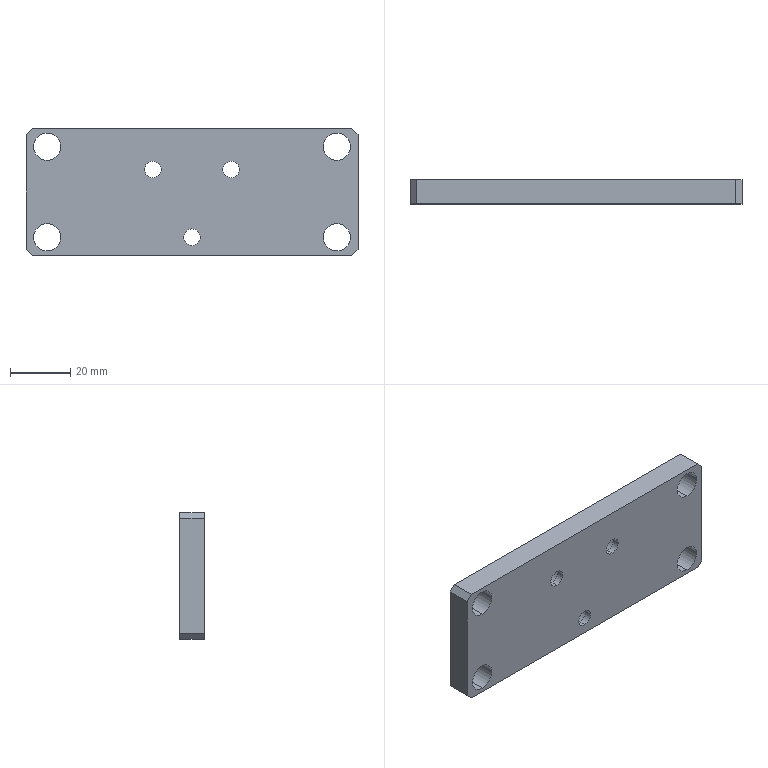Part | SolidWorks | features HoleWzd 2, MirrorPattern 2, Chamfer 1, Extrusion 1 | 1 solid | 33 faces | box 110 x 8 x 42 mm | volume 33353 mm3 | cylinder 20 | plane 13 | commonest cylinder face diameters 9 x8 5.5 x6 10 x6
STEP:
#1=CARTESIAN_POINT('',(-48.,4.,-10.5));
#2=VERTEX_POINT('',#1);
#3=CARTESIAN_POINT('',(-48.,4.,-19.5));
#4=VERTEX_POINT('',#3);
#5=CARTESIAN_POINT('',(-48.,4.,-15.));
#6=DIRECTION('',(0.,-1.,0.));
#7=DIRECTION('',(0.,0.,-1.));
#8=AXIS2_PLACEMENT_3D('',#5,#6,#7);
#9=CIRCLE('',#8,4.5);
#10=EDGE_CURVE('',#2,#4,#9,.T.);
#11=ORIENTED_EDGE('',*,*,#10,.F.);
#12=CARTESIAN_POINT('',(-48.,-4.,-10.5));
#13=VERTEX_POINT('',#12);
#14=CARTESIAN_POINT('',(-48.,-4.,-10.5));
#15=DIRECTION('',(0.,-1.,0.));
#16=VECTOR('',#15,1000.);
#17=LINE('',#14,#16);
#18=EDGE_CURVE('',#2,#13,#17,.T.);
#19=ORIENTED_EDGE('',*,*,#18,.T.);
#20=CARTESIAN_POINT('',(-48.,-4.,-19.5));
#21=VERTEX_POINT('',#20);
#22=CARTESIAN_POINT('',(-48.,-4.,-15.));
#23=DIRECTION('',(0.,-1.,0.));
#24=DIRECTION('',(0.,0.,-1.));
#25=AXIS2_PLACEMENT_3D('',#22,#23,#24);
#26=CIRCLE('',#25,4.5);
#27=EDGE_CURVE('',#13,#21,#26,.T.);
#28=ORIENTED_EDGE('',*,*,#27,.T.);
#29=CARTESIAN_POINT('',(-48.,-4.,-19.5));
#30=DIRECTION('',(0.,-1.,0.));
#31=VECTOR('',#30,1000.);
#32=LINE('',#29,#31);
#33=EDGE_CURVE('',#4,#21,#32,.T.);
#34=ORIENTED_EDGE('',*,*,#33,.F.);
#35=EDGE_LOOP('',(#11,#19,#28,#34));
#36=FACE_OUTER_BOUND('',#35,.T.);
#37=CARTESIAN_POINT('',(-48.,-4.,-15.));
#38=DIRECTION('',(0.,-1.,0.));
#39=DIRECTION('',(0.,0.,-1.));
#40=AXIS2_PLACEMENT_3D('',#37,#38,#39);
#41=CYLINDRICAL_SURFACE('',#40,4.5);
#42=ADVANCED_FACE('',(#36),#41,.F.);
#43=CARTESIAN_POINT('',(-48.,4.,19.5));
#44=VERTEX_POINT('',#43);
#45=CARTESIAN_POINT('',(-48.,4.,10.5));
#46=VERTEX_POINT('',#45);
#47=CARTESIAN_POINT('',(-48.,4.,15.));
#48=DIRECTION('',(0.,-1.,0.));
#49=DIRECTION('',(0.,0.,-1.));
#50=AXIS2_PLACEMENT_3D('',#47,#48,#49);
#51=CIRCLE('',#50,4.5);
#52=EDGE_CURVE('',#44,#46,#51,.T.);
#53=ORIENTED_EDGE('',*,*,#52,.F.);
#54=CARTESIAN_POINT('',(-48.,-4.,19.5));
#55=VERTEX_POINT('',#54);
#56=CARTESIAN_POINT('',(-48.,-4.,19.5));
#57=DIRECTION('',(0.,-1.,0.));
#58=VECTOR('',#57,1000.);
#59=LINE('',#56,#58);
#60=EDGE_CURVE('',#44,#55,#59,.T.);
#61=ORIENTED_EDGE('',*,*,#60,.T.);
#62=CARTESIAN_POINT('',(-48.,-4.,10.5));
#63=VERTEX_POINT('',#62);
#64=CARTESIAN_POINT('',(-48.,-4.,15.));
#65=DIRECTION('',(0.,-1.,0.));
#66=DIRECTION('',(0.,0.,-1.));
#67=AXIS2_PLACEMENT_3D('',#64,#65,#66);
#68=CIRCLE('',#67,4.5);
#69=EDGE_CURVE('',#55,#63,#68,.T.);
#70=ORIENTED_EDGE('',*,*,#69,.T.);
#71=CARTESIAN_POINT('',(-48.,-4.,10.5));
#72=DIRECTION('',(0.,-1.,0.));
#73=VECTOR('',#72,1000.);
#74=LINE('',#71,#73);
#75=EDGE_CURVE('',#46,#63,#74,.T.);
#76=ORIENTED_EDGE('',*,*,#75,.F.);
#77=EDGE_LOOP('',(#53,#61,#70,#76));
#78=FACE_OUTER_BOUND('',#77,.T.);
#79=CARTESIAN_POINT('',(-48.,-4.,15.));
#80=DIRECTION('',(0.,-1.,0.));
#81=DIRECTION('',(0.,0.,-1.));
#82=AXIS2_PLACEMENT_3D('',#79,#80,#81);
#83=CYLINDRICAL_SURFACE('',#82,4.5);
#84=ADVANCED_FACE('',(#78),#83,.F.);
#85=CARTESIAN_POINT('',(48.,4.,-10.5));
#86=VERTEX_POINT('',#85);
#87=CARTESIAN_POINT('',(48.,4.,-19.5));
#88=VERTEX_POINT('',#87);
#89=CARTESIAN_POINT('',(48.,4.,-15.));
#90=DIRECTION('',(0.,-1.,0.));
#91=DIRECTION('',(0.,0.,-1.));
#92=AXIS2_PLACEMENT_3D('',#89,#90,#91);
#93=CIRCLE('',#92,4.5);
#94=EDGE_CURVE('',#86,#88,#93,.T.);
#95=ORIENTED_EDGE('',*,*,#94,.F.);
#96=CARTESIAN_POINT('',(48.,-4.,-10.5));
#97=VERTEX_POINT('',#96);
#98=CARTESIAN_POINT('',(48.,-4.,-10.5));
#99=DIRECTION('',(0.,-1.,0.));
#100=VECTOR('',#99,1000.);
#101=LINE('',#98,#100);
#102=EDGE_CURVE('',#86,#97,#101,.T.);
#103=ORIENTED_EDGE('',*,*,#102,.T.);
#104=CARTESIAN_POINT('',(48.,-4.,-19.5));
#105=VERTEX_POINT('',#104);
#106=CARTESIAN_POINT('',(48.,-4.,-15.));
#107=DIRECTION('',(0.,-1.,0.));
#108=DIRECTION('',(0.,0.,-1.));
#109=AXIS2_PLACEMENT_3D('',#106,#107,#108);
#110=CIRCLE('',#109,4.5);
#111=EDGE_CURVE('',#97,#105,#110,.T.);
#112=ORIENTED_EDGE('',*,*,#111,.T.);
#113=CARTESIAN_POINT('',(48.,-4.,-19.5));
#114=DIRECTION('',(0.,-1.,0.));
#115=VECTOR('',#114,1000.);
#116=LINE('',#113,#115);
#117=EDGE_CURVE('',#88,#105,#116,.T.);
#118=ORIENTED_EDGE('',*,*,#117,.F.);
#119=EDGE_LOOP('',(#95,#103,#112,#118));
#120=FACE_OUTER_BOUND('',#119,.T.);
#121=CARTESIAN_POINT('',(48.,-4.,-15.));
#122=DIRECTION('',(0.,-1.,0.));
#123=DIRECTION('',(0.,0.,-1.));
#124=AXIS2_PLACEMENT_3D('',#121,#122,#123);
#125=CYLINDRICAL_SURFACE('',#124,4.5);
#126=ADVANCED_FACE('',(#120),#125,.F.);
#127=CARTESIAN_POINT('',(48.,4.,19.5));
#128=VERTEX_POINT('',#127);
#129=CARTESIAN_POINT('',(48.,4.,10.5));
#130=VERTEX_POINT('',#129);
#131=CARTESIAN_POINT('',(48.,4.,15.));
#132=DIRECTION('',(0.,-1.,0.));
#133=DIRECTION('',(0.,0.,-1.));
#134=AXIS2_PLACEMENT_3D('',#131,#132,#133);
#135=CIRCLE('',#134,4.5);
#136=EDGE_CURVE('',#128,#130,#135,.T.);
#137=ORIENTED_EDGE('',*,*,#136,.F.);
#138=CARTESIAN_POINT('',(48.,-4.,19.5));
#139=VERTEX_POINT('',#138);
#140=CARTESIAN_POINT('',(48.,-4.,19.5));
#141=DIRECTION('',(0.,-1.,0.));
#142=VECTOR('',#141,1000.);
#143=LINE('',#140,#142);
#144=EDGE_CURVE('',#128,#139,#143,.T.);
#145=ORIENTED_EDGE('',*,*,#144,.T.);
#146=CARTESIAN_POINT('',(48.,-4.,10.5));
#147=VERTEX_POINT('',#146);
#148=CARTESIAN_POINT('',(48.,-4.,15.));
#149=DIRECTION('',(0.,-1.,0.));
#150=DIRECTION('',(0.,0.,-1.));
#151=AXIS2_PLACEMENT_3D('',#148,#149,#150);
#152=CIRCLE('',#151,4.5);
#153=EDGE_CURVE('',#139,#147,#152,.T.);
#154=ORIENTED_EDGE('',*,*,#153,.T.);
#155=CARTESIAN_POINT('',(48.,-4.,10.5));
#156=DIRECTION('',(0.,-1.,0.));
#157=VECTOR('',#156,1000.);
#158=LINE('',#155,#157);
#159=EDGE_CURVE('',#130,#147,#158,.T.);
#160=ORIENTED_EDGE('',*,*,#159,.F.);
#161=EDGE_LOOP('',(#137,#145,#154,#160));
#162=FACE_OUTER_BOUND('',#161,.T.);
#163=CARTESIAN_POINT('',(48.,-4.,15.));
#164=DIRECTION('',(0.,-1.,0.));
#165=DIRECTION('',(0.,0.,-1.));
#166=AXIS2_PLACEMENT_3D('',#163,#164,#165);
#167=CYLINDRICAL_SURFACE('',#166,4.5);
#168=ADVANCED_FACE('',(#162),#167,.F.);
#169=CARTESIAN_POINT('',(0.,-1.7,-20.));
#170=VERTEX_POINT('',#169);
#171=CARTESIAN_POINT('',(0.,-1.7,-10.));
#172=VERTEX_POINT('',#171);
#173=CARTESIAN_POINT('',(0.,-1.7,-15.));
#174=DIRECTION('',(0.,1.,0.));
#175=DIRECTION('',(0.,0.,1.));
#176=AXIS2_PLACEMENT_3D('',#173,#174,#175);
#177=CIRCLE('',#176,5.);
#178=EDGE_CURVE('',#170,#172,#177,.T.);
#179=ORIENTED_EDGE('',*,*,#178,.F.);
#180=CARTESIAN_POINT('',(0.,4.,-20.));
#181=VERTEX_POINT('',#180);
#182=CARTESIAN_POINT('',(0.,4.,-20.));
#183=DIRECTION('',(0.,1.,0.));
#184=VECTOR('',#183,1000.);
#185=LINE('',#182,#184);
#186=EDGE_CURVE('',#170,#181,#185,.T.);
#187=ORIENTED_EDGE('',*,*,#186,.T.);
#188=CARTESIAN_POINT('',(0.,4.,-10.));
#189=VERTEX_POINT('',#188);
#190=CARTESIAN_POINT('',(0.,4.,-15.));
#191=DIRECTION('',(0.,1.,0.));
#192=DIRECTION('',(0.,0.,1.));
#193=AXIS2_PLACEMENT_3D('',#190,#191,#192);
#194=CIRCLE('',#193,5.);
#195=EDGE_CURVE('',#181,#189,#194,.T.);
#196=ORIENTED_EDGE('',*,*,#195,.T.);
#197=CARTESIAN_POINT('',(0.,4.,-10.));
#198=DIRECTION('',(0.,1.,0.));
#199=VECTOR('',#198,1000.);
#200=LINE('',#197,#199);
#201=EDGE_CURVE('',#172,#189,#200,.T.);
#202=ORIENTED_EDGE('',*,*,#201,.F.);
#203=EDGE_LOOP('',(#179,#187,#196,#202));
#204=FACE_OUTER_BOUND('',#203,.T.);
#205=CARTESIAN_POINT('',(0.,4.,-15.));
#206=DIRECTION('',(0.,1.,0.));
#207=DIRECTION('',(0.,0.,1.));
#208=AXIS2_PLACEMENT_3D('',#205,#206,#207);
#209=CYLINDRICAL_SURFACE('',#208,5.);
#210=ADVANCED_FACE('',(#204),#209,.F.);
#211=CARTESIAN_POINT('',(0.,-4.,-17.75));
#212=VERTEX_POINT('',#211);
#213=CARTESIAN_POINT('',(0.,-4.,-12.25));
#214=VERTEX_POINT('',#213);
#215=CARTESIAN_POINT('',(0.,-4.,-15.));
#216=DIRECTION('',(0.,1.,0.));
#217=DIRECTION('',(0.,0.,1.));
#218=AXIS2_PLACEMENT_3D('',#215,#216,#217);
#219=CIRCLE('',#218,2.75);
#220=EDGE_CURVE('',#212,#214,#219,.T.);
#221=ORIENTED_EDGE('',*,*,#220,.F.);
#222=CARTESIAN_POINT('',(0.,-1.7,-17.75));
#223=VERTEX_POINT('',#222);
#224=CARTESIAN_POINT('',(0.,4.,-17.75));
#225=DIRECTION('',(0.,1.,0.));
#226=VECTOR('',#225,1000.);
#227=LINE('',#224,#226);
#228=EDGE_CURVE('',#212,#223,#227,.T.);
#229=ORIENTED_EDGE('',*,*,#228,.T.);
#230=CARTESIAN_POINT('',(0.,-1.7,-12.25));
#231=VERTEX_POINT('',#230);
#232=CARTESIAN_POINT('',(0.,-1.7,-15.));
#233=DIRECTION('',(0.,1.,0.));
#234=DIRECTION('',(0.,0.,1.));
#235=AXIS2_PLACEMENT_3D('',#232,#233,#234);
#236=CIRCLE('',#235,2.75);
#237=EDGE_CURVE('',#223,#231,#236,.T.);
#238=ORIENTED_EDGE('',*,*,#237,.T.);
#239=CARTESIAN_POINT('',(0.,4.,-12.25));
#240=DIRECTION('',(0.,1.,0.));
#241=VECTOR('',#240,1000.);
#242=LINE('',#239,#241);
#243=EDGE_CURVE('',#214,#231,#242,.T.);
#244=ORIENTED_EDGE('',*,*,#243,.F.);
#245=EDGE_LOOP('',(#221,#229,#238,#244));
#246=FACE_OUTER_BOUND('',#245,.T.);
#247=CARTESIAN_POINT('',(0.,4.,-15.));
#248=DIRECTION('',(0.,1.,0.));
#249=DIRECTION('',(0.,0.,1.));
#250=AXIS2_PLACEMENT_3D('',#247,#248,#249);
#251=CYLINDRICAL_SURFACE('',#250,2.75);
#252=ADVANCED_FACE('',(#246),#251,.F.);
#253=CARTESIAN_POINT('',(-12.99,-1.7,2.5));
#254=VERTEX_POINT('',#253);
#255=CARTESIAN_POINT('',(-12.99,-1.7,12.5));
#256=VERTEX_POINT('',#255);
#257=CARTESIAN_POINT('',(-12.99,-1.7,7.5));
#258=DIRECTION('',(0.,1.,0.));
#259=DIRECTION('',(0.,0.,1.));
#260=AXIS2_PLACEMENT_3D('',#257,#258,#259);
#261=CIRCLE('',#260,5.);
#262=EDGE_CURVE('',#254,#256,#261,.T.);
#263=ORIENTED_EDGE('',*,*,#262,.F.);
#264=CARTESIAN_POINT('',(-12.99,4.,2.5));
#265=VERTEX_POINT('',#264);
#266=CARTESIAN_POINT('',(-12.99,4.,2.5));
#267=DIRECTION('',(0.,1.,0.));
#268=VECTOR('',#267,1000.);
#269=LINE('',#266,#268);
#270=EDGE_CURVE('',#254,#265,#269,.T.);
#271=ORIENTED_EDGE('',*,*,#270,.T.);
#272=CARTESIAN_POINT('',(-12.99,4.,12.5));
#273=VERTEX_POINT('',#272);
#274=CARTESIAN_POINT('',(-12.99,4.,7.5));
#275=DIRECTION('',(0.,1.,0.));
#276=DIRECTION('',(0.,0.,1.));
#277=AXIS2_PLACEMENT_3D('',#274,#275,#276);
#278=CIRCLE('',#277,5.);
#279=EDGE_CURVE('',#265,#273,#278,.T.);
#280=ORIENTED_EDGE('',*,*,#279,.T.);
#281=CARTESIAN_POINT('',(-12.99,4.,12.5));
#282=DIRECTION('',(0.,1.,0.));
#283=VECTOR('',#282,1000.);
#284=LINE('',#281,#283);
#285=EDGE_CURVE('',#256,#273,#284,.T.);
#286=ORIENTED_EDGE('',*,*,#285,.F.);
#287=EDGE_LOOP('',(#263,#271,#280,#286));
#288=FACE_OUTER_BOUND('',#287,.T.);
#289=CARTESIAN_POINT('',(-12.99,4.,7.5));
#290=DIRECTION('',(0.,1.,0.));
#291=DIRECTION('',(0.,0.,1.));
#292=AXIS2_PLACEMENT_3D('',#289,#290,#291);
#293=CYLINDRICAL_SURFACE('',#292,5.);
#294=ADVANCED_FACE('',(#288),#293,.F.);
#295=CARTESIAN_POINT('',(-12.99,-4.,4.75));
#296=VERTEX_POINT('',#295);
#297=CARTESIAN_POINT('',(-12.99,-4.,10.25));
#298=VERTEX_POINT('',#297);
#299=CARTESIAN_POINT('',(-12.99,-4.,7.5));
#300=DIRECTION('',(0.,1.,0.));
#301=DIRECTION('',(0.,0.,1.));
#302=AXIS2_PLACEMENT_3D('',#299,#300,#301);
#303=CIRCLE('',#302,2.75);
#304=EDGE_CURVE('',#296,#298,#303,.T.);
#305=ORIENTED_EDGE('',*,*,#304,.F.);
#306=CARTESIAN_POINT('',(-12.99,-1.7,4.75));
#307=VERTEX_POINT('',#306);
#308=CARTESIAN_POINT('',(-12.99,4.,4.75));
#309=DIRECTION('',(0.,1.,0.));
#310=VECTOR('',#309,1000.);
#311=LINE('',#308,#310);
#312=EDGE_CURVE('',#296,#307,#311,.T.);
#313=ORIENTED_EDGE('',*,*,#312,.T.);
#314=CARTESIAN_POINT('',(-12.99,-1.7,10.25));
#315=VERTEX_POINT('',#314);
#316=CARTESIAN_POINT('',(-12.99,-1.7,7.5));
#317=DIRECTION('',(0.,1.,0.));
#318=DIRECTION('',(0.,0.,1.));
#319=AXIS2_PLACEMENT_3D('',#316,#317,#318);
#320=CIRCLE('',#319,2.75);
#321=EDGE_CURVE('',#307,#315,#320,.T.);
#322=ORIENTED_EDGE('',*,*,#321,.T.);
#323=CARTESIAN_POINT('',(-12.99,4.,10.25));
#324=DIRECTION('',(0.,1.,0.));
#325=VECTOR('',#324,1000.);
#326=LINE('',#323,#325);
#327=EDGE_CURVE('',#298,#315,#326,.T.);
#328=ORIENTED_EDGE('',*,*,#327,.F.);
#329=EDGE_LOOP('',(#305,#313,#322,#328));
#330=FACE_OUTER_BOUND('',#329,.T.);
#331=CARTESIAN_POINT('',(-12.99,4.,7.5));
#332=DIRECTION('',(0.,1.,0.));
#333=DIRECTION('',(0.,0.,1.));
#334=AXIS2_PLACEMENT_3D('',#331,#332,#333);
#335=CYLINDRICAL_SURFACE('',#334,2.75);
#336=ADVANCED_FACE('',(#330),#335,.F.);
#337=CARTESIAN_POINT('',(12.99,-1.7,2.5));
#338=VERTEX_POINT('',#337);
#339=CARTESIAN_POINT('',(12.99,-1.7,12.5));
#340=VERTEX_POINT('',#339);
#341=CARTESIAN_POINT('',(12.99,-1.7,7.5));
#342=DIRECTION('',(0.,1.,0.));
#343=DIRECTION('',(0.,0.,1.));
#344=AXIS2_PLACEMENT_3D('',#341,#342,#343);
#345=CIRCLE('',#344,5.);
#346=EDGE_CURVE('',#338,#340,#345,.T.);
#347=ORIENTED_EDGE('',*,*,#346,.F.);
#348=CARTESIAN_POINT('',(12.99,4.,2.5));
#349=VERTEX_POINT('',#348);
#350=CARTESIAN_POINT('',(12.99,4.,2.5));
#351=DIRECTION('',(0.,1.,0.));
#352=VECTOR('',#351,1000.);
#353=LINE('',#350,#352);
#354=EDGE_CURVE('',#338,#349,#353,.T.);
#355=ORIENTED_EDGE('',*,*,#354,.T.);
#356=CARTESIAN_POINT('',(12.99,4.,12.5));
#357=VERTEX_POINT('',#356);
#358=CARTESIAN_POINT('',(12.99,4.,7.5));
#359=DIRECTION('',(0.,1.,0.));
#360=DIRECTION('',(0.,0.,1.));
#361=AXIS2_PLACEMENT_3D('',#358,#359,#360);
#362=CIRCLE('',#361,5.);
#363=EDGE_CURVE('',#349,#357,#362,.T.);
#364=ORIENTED_EDGE('',*,*,#363,.T.);
#365=CARTESIAN_POINT('',(12.99,4.,12.5));
#366=DIRECTION('',(0.,1.,0.));
#367=VECTOR('',#366,1000.);
#368=LINE('',#365,#367);
#369=EDGE_CURVE('',#340,#357,#368,.T.);
#370=ORIENTED_EDGE('',*,*,#369,.F.);
#371=EDGE_LOOP('',(#347,#355,#364,#370));
#372=FACE_OUTER_BOUND('',#371,.T.);
#373=CARTESIAN_POINT('',(12.99,4.,7.5));
#374=DIRECTION('',(0.,1.,0.));
#375=DIRECTION('',(0.,0.,1.));
#376=AXIS2_PLACEMENT_3D('',#373,#374,#375);
#377=CYLINDRICAL_SURFACE('',#376,5.);
#378=ADVANCED_FACE('',(#372),#377,.F.);
#379=CARTESIAN_POINT('',(12.99,-4.,4.75));
#380=VERTEX_POINT('',#379);
#381=CARTESIAN_POINT('',(12.99,-4.,10.25));
#382=VERTEX_POINT('',#381);
#383=CARTESIAN_POINT('',(12.99,-4.,7.5));
#384=DIRECTION('',(0.,1.,0.));
#385=DIRECTION('',(0.,0.,1.));
#386=AXIS2_PLACEMENT_3D('',#383,#384,#385);
#387=CIRCLE('',#386,2.75);
#388=EDGE_CURVE('',#380,#382,#387,.T.);
#389=ORIENTED_EDGE('',*,*,#388,.F.);
#390=CARTESIAN_POINT('',(12.99,-1.7,4.75));
#391=VERTEX_POINT('',#390);
#392=CARTESIAN_POINT('',(12.99,4.,4.75));
#393=DIRECTION('',(0.,1.,0.));
#394=VECTOR('',#393,1000.);
#395=LINE('',#392,#394);
#396=EDGE_CURVE('',#380,#391,#395,.T.);
#397=ORIENTED_EDGE('',*,*,#396,.T.);
#398=CARTESIAN_POINT('',(12.99,-1.7,10.25));
#399=VERTEX_POINT('',#398);
#400=CARTESIAN_POINT('',(12.99,-1.7,7.5));
#401=DIRECTION('',(0.,1.,0.));
#402=DIRECTION('',(0.,0.,1.));
#403=AXIS2_PLACEMENT_3D('',#400,#401,#402);
#404=CIRCLE('',#403,2.75);
#405=EDGE_CURVE('',#391,#399,#404,.T.);
#406=ORIENTED_EDGE('',*,*,#405,.T.);
#407=CARTESIAN_POINT('',(12.99,4.,10.25));
#408=DIRECTION('',(0.,1.,0.));
#409=VECTOR('',#408,1000.);
#410=LINE('',#407,#409);
#411=EDGE_CURVE('',#382,#399,#410,.T.);
#412=ORIENTED_EDGE('',*,*,#411,.F.);
#413=EDGE_LOOP('',(#389,#397,#406,#412));
#414=FACE_OUTER_BOUND('',#413,.T.);
#415=CARTESIAN_POINT('',(12.99,4.,7.5));
#416=DIRECTION('',(0.,1.,0.));
#417=DIRECTION('',(0.,0.,1.));
#418=AXIS2_PLACEMENT_3D('',#415,#416,#417);
#419=CYLINDRICAL_SURFACE('',#418,2.75);
#420=ADVANCED_FACE('',(#414),#419,.F.);
#421=CARTESIAN_POINT('',(-48.,-4.,-15.));
#422=DIRECTION('',(0.,-1.,0.));
#423=DIRECTION('',(0.,0.,-1.));
#424=AXIS2_PLACEMENT_3D('',#421,#422,#423);
#425=CIRCLE('',#424,4.5);
#426=EDGE_CURVE('',#21,#13,#425,.T.);
#427=ORIENTED_EDGE('',*,*,#426,.F.);
#428=ORIENTED_EDGE('',*,*,#27,.F.);
#429=EDGE_LOOP('',(#427,#428));
#430=FACE_BOUND('',#429,.T.);
#431=CARTESIAN_POINT('',(-53.,-4.,21.));
#432=VERTEX_POINT('',#431);
#433=CARTESIAN_POINT('',(53.,-4.,21.));
#434=VERTEX_POINT('',#433);
#435=CARTESIAN_POINT('',(-55.,-4.,21.));
#436=DIRECTION('',(1.,0.,0.));
#437=VECTOR('',#436,1000.);
#438=LINE('',#435,#437);
#439=EDGE_CURVE('',#432,#434,#438,.T.);
#440=ORIENTED_EDGE('',*,*,#439,.F.);
#441=CARTESIAN_POINT('',(-55.,-4.,19.));
#442=VERTEX_POINT('',#441);
#443=CARTESIAN_POINT('',(-53.,-4.,21.));
#444=DIRECTION('',(-0.7071,0.,-0.7071));
#445=VECTOR('',#444,1000.);
#446=LINE('',#443,#445);
#447=EDGE_CURVE('',#432,#442,#446,.T.);
#448=ORIENTED_EDGE('',*,*,#447,.T.);
#449=CARTESIAN_POINT('',(-55.,-4.,-19.));
#450=VERTEX_POINT('',#449);
#451=CARTESIAN_POINT('',(-55.,-4.,-21.));
#452=DIRECTION('',(0.,0.,1.));
#453=VECTOR('',#452,1000.);
#454=LINE('',#451,#453);
#455=EDGE_CURVE('',#450,#442,#454,.T.);
#456=ORIENTED_EDGE('',*,*,#455,.F.);
#457=CARTESIAN_POINT('',(-53.,-4.,-21.));
#458=VERTEX_POINT('',#457);
#459=CARTESIAN_POINT('',(-55.,-4.,-19.));
#460=DIRECTION('',(0.7071,0.,-0.7071));
#461=VECTOR('',#460,1000.);
#462=LINE('',#459,#461);
#463=EDGE_CURVE('',#450,#458,#462,.T.);
#464=ORIENTED_EDGE('',*,*,#463,.T.);
#465=CARTESIAN_POINT('',(53.,-4.,-21.));
#466=VERTEX_POINT('',#465);
#467=CARTESIAN_POINT('',(-55.,-4.,-21.));
#468=DIRECTION('',(-1.,0.,0.));
#469=VECTOR('',#468,1000.);
#470=LINE('',#467,#469);
#471=EDGE_CURVE('',#466,#458,#470,.T.);
#472=ORIENTED_EDGE('',*,*,#471,.F.);
#473=CARTESIAN_POINT('',(55.,-4.,-19.));
#474=VERTEX_POINT('',#473);
#475=CARTESIAN_POINT('',(53.,-4.,-21.));
#476=DIRECTION('',(0.7071,0.,0.7071));
#477=VECTOR('',#476,1000.);
#478=LINE('',#475,#477);
#479=EDGE_CURVE('',#466,#474,#478,.T.);
#480=ORIENTED_EDGE('',*,*,#479,.T.);
#481=CARTESIAN_POINT('',(55.,-4.,19.));
#482=VERTEX_POINT('',#481);
#483=CARTESIAN_POINT('',(55.,-4.,-21.));
#484=DIRECTION('',(0.,0.,-1.));
#485=VECTOR('',#484,1000.);
#486=LINE('',#483,#485);
#487=EDGE_CURVE('',#482,#474,#486,.T.);
#488=ORIENTED_EDGE('',*,*,#487,.F.);
#489=CARTESIAN_POINT('',(55.,-4.,19.));
#490=DIRECTION('',(-0.7071,0.,0.7071));
#491=VECTOR('',#490,1000.);
#492=LINE('',#489,#491);
#493=EDGE_CURVE('',#482,#434,#492,.T.);
#494=ORIENTED_EDGE('',*,*,#493,.T.);
#495=EDGE_LOOP('',(#440,#448,#456,#464,#472,#480,#488,#494));
#496=FACE_OUTER_BOUND('',#495,.T.);
#497=CARTESIAN_POINT('',(12.99,-4.,7.5));
#498=DIRECTION('',(0.,1.,0.));
#499=DIRECTION('',(0.,0.,1.));
#500=AXIS2_PLACEMENT_3D('',#497,#498,#499);
#501=CIRCLE('',#500,2.75);
#502=EDGE_CURVE('',#382,#380,#501,.T.);
#503=ORIENTED_EDGE('',*,*,#502,.T.);
#504=ORIENTED_EDGE('',*,*,#388,.T.);
#505=EDGE_LOOP('',(#503,#504));
#506=FACE_BOUND('',#505,.T.);
#507=CARTESIAN_POINT('',(-12.99,-4.,7.5));
#508=DIRECTION('',(0.,1.,0.));
#509=DIRECTION('',(0.,0.,1.));
#510=AXIS2_PLACEMENT_3D('',#507,#508,#509);
#511=CIRCLE('',#510,2.75);
#512=EDGE_CURVE('',#298,#296,#511,.T.);
#513=ORIENTED_EDGE('',*,*,#512,.T.);
#514=ORIENTED_EDGE('',*,*,#304,.T.);
#515=EDGE_LOOP('',(#513,#514));
#516=FACE_BOUND('',#515,.T.);
#517=CARTESIAN_POINT('',(0.,-4.,-15.));
#518=DIRECTION('',(0.,1.,0.));
#519=DIRECTION('',(0.,0.,1.));
#520=AXIS2_PLACEMENT_3D('',#517,#518,#519);
#521=CIRCLE('',#520,2.75);
#522=EDGE_CURVE('',#214,#212,#521,.T.);
#523=ORIENTED_EDGE('',*,*,#522,.T.);
#524=ORIENTED_EDGE('',*,*,#220,.T.);
#525=EDGE_LOOP('',(#523,#524));
#526=FACE_BOUND('',#525,.T.);
#527=CARTESIAN_POINT('',(48.,-4.,15.));
#528=DIRECTION('',(0.,-1.,0.));
#529=DIRECTION('',(0.,0.,-1.));
#530=AXIS2_PLACEMENT_3D('',#527,#528,#529);
#531=CIRCLE('',#530,4.5);
#532=EDGE_CURVE('',#147,#139,#531,.T.);
#533=ORIENTED_EDGE('',*,*,#532,.F.);
#534=ORIENTED_EDGE('',*,*,#153,.F.);
#535=EDGE_LOOP('',(#533,#534));
#536=FACE_BOUND('',#535,.T.);
#537=CARTESIAN_POINT('',(48.,-4.,-15.));
#538=DIRECTION('',(0.,-1.,0.));
#539=DIRECTION('',(0.,0.,-1.));
#540=AXIS2_PLACEMENT_3D('',#537,#538,#539);
#541=CIRCLE('',#540,4.5);
#542=EDGE_CURVE('',#105,#97,#541,.T.);
#543=ORIENTED_EDGE('',*,*,#542,.F.);
#544=ORIENTED_EDGE('',*,*,#111,.F.);
#545=EDGE_LOOP('',(#543,#544));
#546=FACE_BOUND('',#545,.T.);
#547=CARTESIAN_POINT('',(-48.,-4.,15.));
#548=DIRECTION('',(0.,-1.,0.));
#549=DIRECTION('',(0.,0.,-1.));
#550=AXIS2_PLACEMENT_3D('',#547,#548,#549);
#551=CIRCLE('',#550,4.5);
#552=EDGE_CURVE('',#63,#55,#551,.T.);
#553=ORIENTED_EDGE('',*,*,#552,.F.);
#554=ORIENTED_EDGE('',*,*,#69,.F.);
#555=EDGE_LOOP('',(#553,#554));
#556=FACE_BOUND('',#555,.T.);
#557=CARTESIAN_POINT('',(0.,-4.,0.));
#558=DIRECTION('',(0.,1.,0.));
#559=DIRECTION('',(0.,0.,1.));
#560=AXIS2_PLACEMENT_3D('',#557,#558,#559);
#561=PLANE('',#560);
#562=ADVANCED_FACE('',(#430,#496,#506,#516,#526,#536,#546,#556),#561,.F.);
#563=CARTESIAN_POINT('',(-48.,4.,-15.));
#564=DIRECTION('',(0.,-1.,0.));
#565=DIRECTION('',(0.,0.,-1.));
#566=AXIS2_PLACEMENT_3D('',#563,#564,#565);
#567=CIRCLE('',#566,4.5);
#568=EDGE_CURVE('',#4,#2,#567,.T.);
#569=ORIENTED_EDGE('',*,*,#568,.T.);
#570=ORIENTED_EDGE('',*,*,#10,.T.);
#571=EDGE_LOOP('',(#569,#570));
#572=FACE_BOUND('',#571,.T.);
#573=CARTESIAN_POINT('',(-55.,4.,-19.));
#574=VERTEX_POINT('',#573);
#575=CARTESIAN_POINT('',(-55.,4.,19.));
#576=VERTEX_POINT('',#575);
#577=CARTESIAN_POINT('',(-55.,4.,-21.));
#578=DIRECTION('',(0.,0.,1.));
#579=VECTOR('',#578,1000.);
#580=LINE('',#577,#579);
#581=EDGE_CURVE('',#574,#576,#580,.T.);
#582=ORIENTED_EDGE('',*,*,#581,.T.);
#583=CARTESIAN_POINT('',(-53.,4.,21.));
#584=VERTEX_POINT('',#583);
#585=CARTESIAN_POINT('',(-37.,4.,37.));
#586=DIRECTION('',(0.7071,0.,0.7071));
#587=VECTOR('',#586,1000.);
#588=LINE('',#585,#587);
#589=EDGE_CURVE('',#576,#584,#588,.T.);
#590=ORIENTED_EDGE('',*,*,#589,.T.);
#591=CARTESIAN_POINT('',(53.,4.,21.));
#592=VERTEX_POINT('',#591);
#593=CARTESIAN_POINT('',(-55.,4.,21.));
#594=DIRECTION('',(1.,0.,0.));
#595=VECTOR('',#594,1000.);
#596=LINE('',#593,#595);
#597=EDGE_CURVE('',#584,#592,#596,.T.);
#598=ORIENTED_EDGE('',*,*,#597,.T.);
#599=CARTESIAN_POINT('',(55.,4.,19.));
#600=VERTEX_POINT('',#599);
#601=CARTESIAN_POINT('',(37.,4.,37.));
#602=DIRECTION('',(0.7071,0.,-0.7071));
#603=VECTOR('',#602,1000.);
#604=LINE('',#601,#603);
#605=EDGE_CURVE('',#592,#600,#604,.T.);
#606=ORIENTED_EDGE('',*,*,#605,.T.);
#607=CARTESIAN_POINT('',(55.,4.,-19.));
#608=VERTEX_POINT('',#607);
#609=CARTESIAN_POINT('',(55.,4.,-21.));
#610=DIRECTION('',(0.,0.,-1.));
#611=VECTOR('',#610,1000.);
#612=LINE('',#609,#611);
#613=EDGE_CURVE('',#600,#608,#612,.T.);
#614=ORIENTED_EDGE('',*,*,#613,.T.);
#615=CARTESIAN_POINT('',(53.,4.,-21.));
#616=VERTEX_POINT('',#615);
#617=CARTESIAN_POINT('',(37.,4.,-37.));
#618=DIRECTION('',(-0.7071,0.,-0.7071));
#619=VECTOR('',#618,1000.);
#620=LINE('',#617,#619);
#621=EDGE_CURVE('',#608,#616,#620,.T.);
#622=ORIENTED_EDGE('',*,*,#621,.T.);
#623=CARTESIAN_POINT('',(-53.,4.,-21.));
#624=VERTEX_POINT('',#623);
#625=CARTESIAN_POINT('',(-55.,4.,-21.));
#626=DIRECTION('',(-1.,0.,0.));
#627=VECTOR('',#626,1000.);
#628=LINE('',#625,#627);
#629=EDGE_CURVE('',#616,#624,#628,.T.);
#630=ORIENTED_EDGE('',*,*,#629,.T.);
#631=CARTESIAN_POINT('',(-37.,4.,-37.));
#632=DIRECTION('',(-0.7071,0.,0.7071));
#633=VECTOR('',#632,1000.);
#634=LINE('',#631,#633);
#635=EDGE_CURVE('',#624,#574,#634,.T.);
#636=ORIENTED_EDGE('',*,*,#635,.T.);
#637=EDGE_LOOP('',(#582,#590,#598,#606,#614,#622,#630,#636));
#638=FACE_OUTER_BOUND('',#637,.T.);
#639=CARTESIAN_POINT('',(12.99,4.,7.5));
#640=DIRECTION('',(0.,1.,0.));
#641=DIRECTION('',(0.,0.,1.));
#642=AXIS2_PLACEMENT_3D('',#639,#640,#641);
#643=CIRCLE('',#642,5.);
#644=EDGE_CURVE('',#357,#349,#643,.T.);
#645=ORIENTED_EDGE('',*,*,#644,.F.);
#646=ORIENTED_EDGE('',*,*,#363,.F.);
#647=EDGE_LOOP('',(#645,#646));
#648=FACE_BOUND('',#647,.T.);
#649=CARTESIAN_POINT('',(-12.99,4.,7.5));
#650=DIRECTION('',(0.,1.,0.));
#651=DIRECTION('',(0.,0.,1.));
#652=AXIS2_PLACEMENT_3D('',#649,#650,#651);
#653=CIRCLE('',#652,5.);
#654=EDGE_CURVE('',#273,#265,#653,.T.);
#655=ORIENTED_EDGE('',*,*,#654,.F.);
#656=ORIENTED_EDGE('',*,*,#279,.F.);
#657=EDGE_LOOP('',(#655,#656));
#658=FACE_BOUND('',#657,.T.);
#659=CARTESIAN_POINT('',(0.,4.,-15.));
#660=DIRECTION('',(0.,1.,0.));
#661=DIRECTION('',(0.,0.,1.));
#662=AXIS2_PLACEMENT_3D('',#659,#660,#661);
#663=CIRCLE('',#662,5.);
#664=EDGE_CURVE('',#189,#181,#663,.T.);
#665=ORIENTED_EDGE('',*,*,#664,.F.);
#666=ORIENTED_EDGE('',*,*,#195,.F.);
#667=EDGE_LOOP('',(#665,#666));
#668=FACE_BOUND('',#667,.T.);
#669=CARTESIAN_POINT('',(48.,4.,15.));
#670=DIRECTION('',(0.,-1.,0.));
#671=DIRECTION('',(0.,0.,-1.));
#672=AXIS2_PLACEMENT_3D('',#669,#670,#671);
#673=CIRCLE('',#672,4.5);
#674=EDGE_CURVE('',#130,#128,#673,.T.);
#675=ORIENTED_EDGE('',*,*,#674,.T.);
#676=ORIENTED_EDGE('',*,*,#136,.T.);
#677=EDGE_LOOP('',(#675,#676));
#678=FACE_BOUND('',#677,.T.);
#679=CARTESIAN_POINT('',(48.,4.,-15.));
#680=DIRECTION('',(0.,-1.,0.));
#681=DIRECTION('',(0.,0.,-1.));
#682=AXIS2_PLACEMENT_3D('',#679,#680,#681);
#683=CIRCLE('',#682,4.5);
#684=EDGE_CURVE('',#88,#86,#683,.T.);
#685=ORIENTED_EDGE('',*,*,#684,.T.);
#686=ORIENTED_EDGE('',*,*,#94,.T.);
#687=EDGE_LOOP('',(#685,#686));
#688=FACE_BOUND('',#687,.T.);
#689=CARTESIAN_POINT('',(-48.,4.,15.));
#690=DIRECTION('',(0.,-1.,0.));
#691=DIRECTION('',(0.,0.,-1.));
#692=AXIS2_PLACEMENT_3D('',#689,#690,#691);
#693=CIRCLE('',#692,4.5);
#694=EDGE_CURVE('',#46,#44,#693,.T.);
#695=ORIENTED_EDGE('',*,*,#694,.T.);
#696=ORIENTED_EDGE('',*,*,#52,.T.);
#697=EDGE_LOOP('',(#695,#696));
#698=FACE_BOUND('',#697,.T.);
#699=CARTESIAN_POINT('',(0.,4.,0.));
#700=DIRECTION('',(0.,1.,0.));
#701=DIRECTION('',(0.,0.,1.));
#702=AXIS2_PLACEMENT_3D('',#699,#700,#701);
#703=PLANE('',#702);
#704=ADVANCED_FACE('',(#572,#638,#648,#658,#668,#678,#688,#698),#703,.T.);
#705=ORIENTED_EDGE('',*,*,#613,.F.);
#706=CARTESIAN_POINT('',(55.,4.,19.));
#707=DIRECTION('',(0.,-1.,0.));
#708=VECTOR('',#707,1000.);
#709=LINE('',#706,#708);
#710=EDGE_CURVE('',#600,#482,#709,.T.);
#711=ORIENTED_EDGE('',*,*,#710,.T.);
#712=ORIENTED_EDGE('',*,*,#487,.T.);
#713=CARTESIAN_POINT('',(55.,4.,-19.));
#714=DIRECTION('',(0.,1.,0.));
#715=VECTOR('',#714,1000.);
#716=LINE('',#713,#715);
#717=EDGE_CURVE('',#474,#608,#716,.T.);
#718=ORIENTED_EDGE('',*,*,#717,.T.);
#719=EDGE_LOOP('',(#705,#711,#712,#718));
#720=FACE_OUTER_BOUND('',#719,.T.);
#721=CARTESIAN_POINT('',(55.,4.,-21.));
#722=DIRECTION('',(-1.,0.,0.));
#723=DIRECTION('',(0.,0.,1.));
#724=AXIS2_PLACEMENT_3D('',#721,#722,#723);
#725=PLANE('',#724);
#726=ADVANCED_FACE('',(#720),#725,.F.);
#727=ORIENTED_EDGE('',*,*,#629,.F.);
#728=CARTESIAN_POINT('',(53.,4.,-21.));
#729=DIRECTION('',(0.,-1.,0.));
#730=VECTOR('',#729,1000.);
#731=LINE('',#728,#730);
#732=EDGE_CURVE('',#616,#466,#731,.T.);
#733=ORIENTED_EDGE('',*,*,#732,.T.);
#734=ORIENTED_EDGE('',*,*,#471,.T.);
#735=CARTESIAN_POINT('',(-53.,4.,-21.));
#736=DIRECTION('',(0.,1.,0.));
#737=VECTOR('',#736,1000.);
#738=LINE('',#735,#737);
#739=EDGE_CURVE('',#458,#624,#738,.T.);
#740=ORIENTED_EDGE('',*,*,#739,.T.);
#741=EDGE_LOOP('',(#727,#733,#734,#740));
#742=FACE_OUTER_BOUND('',#741,.T.);
#743=CARTESIAN_POINT('',(-55.,4.,-21.));
#744=DIRECTION('',(0.,0.,1.));
#745=DIRECTION('',(1.,0.,0.));
#746=AXIS2_PLACEMENT_3D('',#743,#744,#745);
#747=PLANE('',#746);
#748=ADVANCED_FACE('',(#742),#747,.F.);
#749=ORIENTED_EDGE('',*,*,#455,.T.);
#750=CARTESIAN_POINT('',(-55.,4.,19.));
#751=DIRECTION('',(0.,1.,0.));
#752=VECTOR('',#751,1000.);
#753=LINE('',#750,#752);
#754=EDGE_CURVE('',#442,#576,#753,.T.);
#755=ORIENTED_EDGE('',*,*,#754,.T.);
#756=ORIENTED_EDGE('',*,*,#581,.F.);
#757=CARTESIAN_POINT('',(-55.,4.,-19.));
#758=DIRECTION('',(0.,-1.,0.));
#759=VECTOR('',#758,1000.);
#760=LINE('',#757,#759);
#761=EDGE_CURVE('',#574,#450,#760,.T.);
#762=ORIENTED_EDGE('',*,*,#761,.T.);
#763=EDGE_LOOP('',(#749,#755,#756,#762));
#764=FACE_OUTER_BOUND('',#763,.T.);
#765=CARTESIAN_POINT('',(-55.,4.,-21.));
#766=DIRECTION('',(1.,0.,0.));
#767=DIRECTION('',(0.,0.,-1.));
#768=AXIS2_PLACEMENT_3D('',#765,#766,#767);
#769=PLANE('',#768);
#770=ADVANCED_FACE('',(#764),#769,.F.);
#771=ORIENTED_EDGE('',*,*,#597,.F.);
#772=CARTESIAN_POINT('',(-53.,4.,21.));
#773=DIRECTION('',(0.,-1.,0.));
#774=VECTOR('',#773,1000.);
#775=LINE('',#772,#774);
#776=EDGE_CURVE('',#584,#432,#775,.T.);
#777=ORIENTED_EDGE('',*,*,#776,.T.);
#778=ORIENTED_EDGE('',*,*,#439,.T.);
#779=CARTESIAN_POINT('',(53.,4.,21.));
#780=DIRECTION('',(0.,1.,0.));
#781=VECTOR('',#780,1000.);
#782=LINE('',#779,#781);
#783=EDGE_CURVE('',#434,#592,#782,.T.);
#784=ORIENTED_EDGE('',*,*,#783,.T.);
#785=EDGE_LOOP('',(#771,#777,#778,#784));
#786=FACE_OUTER_BOUND('',#785,.T.);
#787=CARTESIAN_POINT('',(-55.,4.,21.));
#788=DIRECTION('',(0.,0.,-1.));
#789=DIRECTION('',(-1.,0.,0.));
#790=AXIS2_PLACEMENT_3D('',#787,#788,#789);
#791=PLANE('',#790);
#792=ADVANCED_FACE('',(#786),#791,.F.);
#793=ORIENTED_EDGE('',*,*,#396,.F.);
#794=ORIENTED_EDGE('',*,*,#502,.F.);
#795=ORIENTED_EDGE('',*,*,#411,.T.);
#796=CARTESIAN_POINT('',(12.99,-1.7,7.5));
#797=DIRECTION('',(0.,1.,0.));
#798=DIRECTION('',(0.,0.,1.));
#799=AXIS2_PLACEMENT_3D('',#796,#797,#798);
#800=CIRCLE('',#799,2.75);
#801=EDGE_CURVE('',#399,#391,#800,.T.);
#802=ORIENTED_EDGE('',*,*,#801,.T.);
#803=EDGE_LOOP('',(#793,#794,#795,#802));
#804=FACE_OUTER_BOUND('',#803,.T.);
#805=CARTESIAN_POINT('',(12.99,4.,7.5));
#806=DIRECTION('',(0.,1.,0.));
#807=DIRECTION('',(0.,0.,1.));
#808=AXIS2_PLACEMENT_3D('',#805,#806,#807);
#809=CYLINDRICAL_SURFACE('',#808,2.75);
#810=ADVANCED_FACE('',(#804),#809,.F.);
#811=ORIENTED_EDGE('',*,*,#801,.F.);
#812=ORIENTED_EDGE('',*,*,#405,.F.);
#813=EDGE_LOOP('',(#811,#812));
#814=FACE_BOUND('',#813,.T.);
#815=CARTESIAN_POINT('',(12.99,-1.7,7.5));
#816=DIRECTION('',(0.,1.,0.));
#817=DIRECTION('',(0.,0.,1.));
#818=AXIS2_PLACEMENT_3D('',#815,#816,#817);
#819=CIRCLE('',#818,5.);
#820=EDGE_CURVE('',#340,#338,#819,.T.);
#821=ORIENTED_EDGE('',*,*,#820,.T.);
#822=ORIENTED_EDGE('',*,*,#346,.T.);
#823=EDGE_LOOP('',(#821,#822));
#824=FACE_OUTER_BOUND('',#823,.T.);
#825=CARTESIAN_POINT('',(15.74,-1.7,7.5));
#826=DIRECTION('',(0.,-1.,0.));
#827=DIRECTION('',(0.,0.,-1.));
#828=AXIS2_PLACEMENT_3D('',#825,#826,#827);
#829=PLANE('',#828);
#830=ADVANCED_FACE('',(#814,#824),#829,.F.);
#831=ORIENTED_EDGE('',*,*,#354,.F.);
#832=ORIENTED_EDGE('',*,*,#820,.F.);
#833=ORIENTED_EDGE('',*,*,#369,.T.);
#834=ORIENTED_EDGE('',*,*,#644,.T.);
#835=EDGE_LOOP('',(#831,#832,#833,#834));
#836=FACE_OUTER_BOUND('',#835,.T.);
#837=CARTESIAN_POINT('',(12.99,4.,7.5));
#838=DIRECTION('',(0.,1.,0.));
#839=DIRECTION('',(0.,0.,1.));
#840=AXIS2_PLACEMENT_3D('',#837,#838,#839);
#841=CYLINDRICAL_SURFACE('',#840,5.);
#842=ADVANCED_FACE('',(#836),#841,.F.);
#843=ORIENTED_EDGE('',*,*,#312,.F.);
#844=ORIENTED_EDGE('',*,*,#512,.F.);
#845=ORIENTED_EDGE('',*,*,#327,.T.);
#846=CARTESIAN_POINT('',(-12.99,-1.7,7.5));
#847=DIRECTION('',(0.,1.,0.));
#848=DIRECTION('',(0.,0.,1.));
#849=AXIS2_PLACEMENT_3D('',#846,#847,#848);
#850=CIRCLE('',#849,2.75);
#851=EDGE_CURVE('',#315,#307,#850,.T.);
#852=ORIENTED_EDGE('',*,*,#851,.T.);
#853=EDGE_LOOP('',(#843,#844,#845,#852));
#854=FACE_OUTER_BOUND('',#853,.T.);
#855=CARTESIAN_POINT('',(-12.99,4.,7.5));
#856=DIRECTION('',(0.,1.,0.));
#857=DIRECTION('',(0.,0.,1.));
#858=AXIS2_PLACEMENT_3D('',#855,#856,#857);
#859=CYLINDRICAL_SURFACE('',#858,2.75);
#860=ADVANCED_FACE('',(#854),#859,.F.);
#861=ORIENTED_EDGE('',*,*,#851,.F.);
#862=ORIENTED_EDGE('',*,*,#321,.F.);
#863=EDGE_LOOP('',(#861,#862));
#864=FACE_BOUND('',#863,.T.);
#865=CARTESIAN_POINT('',(-12.99,-1.7,7.5));
#866=DIRECTION('',(0.,1.,0.));
#867=DIRECTION('',(0.,0.,1.));
#868=AXIS2_PLACEMENT_3D('',#865,#866,#867);
#869=CIRCLE('',#868,5.);
#870=EDGE_CURVE('',#256,#254,#869,.T.);
#871=ORIENTED_EDGE('',*,*,#870,.T.);
#872=ORIENTED_EDGE('',*,*,#262,.T.);
#873=EDGE_LOOP('',(#871,#872));
#874=FACE_OUTER_BOUND('',#873,.T.);
#875=CARTESIAN_POINT('',(-10.24,-1.7,7.5));
#876=DIRECTION('',(0.,-1.,0.));
#877=DIRECTION('',(0.,0.,-1.));
#878=AXIS2_PLACEMENT_3D('',#875,#876,#877);
#879=PLANE('',#878);
#880=ADVANCED_FACE('',(#864,#874),#879,.F.);
#881=ORIENTED_EDGE('',*,*,#270,.F.);
#882=ORIENTED_EDGE('',*,*,#870,.F.);
#883=ORIENTED_EDGE('',*,*,#285,.T.);
#884=ORIENTED_EDGE('',*,*,#654,.T.);
#885=EDGE_LOOP('',(#881,#882,#883,#884));
#886=FACE_OUTER_BOUND('',#885,.T.);
#887=CARTESIAN_POINT('',(-12.99,4.,7.5));
#888=DIRECTION('',(0.,1.,0.));
#889=DIRECTION('',(0.,0.,1.));
#890=AXIS2_PLACEMENT_3D('',#887,#888,#889);
#891=CYLINDRICAL_SURFACE('',#890,5.);
#892=ADVANCED_FACE('',(#886),#891,.F.);
#893=ORIENTED_EDGE('',*,*,#228,.F.);
#894=ORIENTED_EDGE('',*,*,#522,.F.);
#895=ORIENTED_EDGE('',*,*,#243,.T.);
#896=CARTESIAN_POINT('',(0.,-1.7,-15.));
#897=DIRECTION('',(0.,1.,0.));
#898=DIRECTION('',(0.,0.,1.));
#899=AXIS2_PLACEMENT_3D('',#896,#897,#898);
#900=CIRCLE('',#899,2.75);
#901=EDGE_CURVE('',#231,#223,#900,.T.);
#902=ORIENTED_EDGE('',*,*,#901,.T.);
#903=EDGE_LOOP('',(#893,#894,#895,#902));
#904=FACE_OUTER_BOUND('',#903,.T.);
#905=CARTESIAN_POINT('',(0.,4.,-15.));
#906=DIRECTION('',(0.,1.,0.));
#907=DIRECTION('',(0.,0.,1.));
#908=AXIS2_PLACEMENT_3D('',#905,#906,#907);
#909=CYLINDRICAL_SURFACE('',#908,2.75);
#910=ADVANCED_FACE('',(#904),#909,.F.);
#911=ORIENTED_EDGE('',*,*,#901,.F.);
#912=ORIENTED_EDGE('',*,*,#237,.F.);
#913=EDGE_LOOP('',(#911,#912));
#914=FACE_BOUND('',#913,.T.);
#915=CARTESIAN_POINT('',(0.,-1.7,-15.));
#916=DIRECTION('',(0.,1.,0.));
#917=DIRECTION('',(0.,0.,1.));
#918=AXIS2_PLACEMENT_3D('',#915,#916,#917);
#919=CIRCLE('',#918,5.);
#920=EDGE_CURVE('',#172,#170,#919,.T.);
#921=ORIENTED_EDGE('',*,*,#920,.T.);
#922=ORIENTED_EDGE('',*,*,#178,.T.);
#923=EDGE_LOOP('',(#921,#922));
#924=FACE_OUTER_BOUND('',#923,.T.);
#925=CARTESIAN_POINT('',(2.75,-1.7,-15.));
#926=DIRECTION('',(0.,-1.,0.));
#927=DIRECTION('',(0.,0.,-1.));
#928=AXIS2_PLACEMENT_3D('',#925,#926,#927);
#929=PLANE('',#928);
#930=ADVANCED_FACE('',(#914,#924),#929,.F.);
#931=ORIENTED_EDGE('',*,*,#186,.F.);
#932=ORIENTED_EDGE('',*,*,#920,.F.);
#933=ORIENTED_EDGE('',*,*,#201,.T.);
#934=ORIENTED_EDGE('',*,*,#664,.T.);
#935=EDGE_LOOP('',(#931,#932,#933,#934));
#936=FACE_OUTER_BOUND('',#935,.T.);
#937=CARTESIAN_POINT('',(0.,4.,-15.));
#938=DIRECTION('',(0.,1.,0.));
#939=DIRECTION('',(0.,0.,1.));
#940=AXIS2_PLACEMENT_3D('',#937,#938,#939);
#941=CYLINDRICAL_SURFACE('',#940,5.);
#942=ADVANCED_FACE('',(#936),#941,.F.);
#943=ORIENTED_EDGE('',*,*,#144,.F.);
#944=ORIENTED_EDGE('',*,*,#674,.F.);
#945=ORIENTED_EDGE('',*,*,#159,.T.);
#946=ORIENTED_EDGE('',*,*,#532,.T.);
#947=EDGE_LOOP('',(#943,#944,#945,#946));
#948=FACE_OUTER_BOUND('',#947,.T.);
#949=CARTESIAN_POINT('',(48.,-4.,15.));
#950=DIRECTION('',(0.,-1.,0.));
#951=DIRECTION('',(0.,0.,-1.));
#952=AXIS2_PLACEMENT_3D('',#949,#950,#951);
#953=CYLINDRICAL_SURFACE('',#952,4.5);
#954=ADVANCED_FACE('',(#948),#953,.F.);
#955=ORIENTED_EDGE('',*,*,#589,.F.);
#956=ORIENTED_EDGE('',*,*,#754,.F.);
#957=ORIENTED_EDGE('',*,*,#447,.F.);
#958=ORIENTED_EDGE('',*,*,#776,.F.);
#959=EDGE_LOOP('',(#955,#956,#957,#958));
#960=FACE_OUTER_BOUND('',#959,.T.);
#961=CARTESIAN_POINT('',(-53.,4.,21.));
#962=DIRECTION('',(0.7071,0.,-0.7071));
#963=DIRECTION('',(0.,-1.,0.));
#964=AXIS2_PLACEMENT_3D('',#961,#962,#963);
#965=PLANE('',#964);
#966=ADVANCED_FACE('',(#960),#965,.F.);
#967=ORIENTED_EDGE('',*,*,#605,.F.);
#968=ORIENTED_EDGE('',*,*,#783,.F.);
#969=ORIENTED_EDGE('',*,*,#493,.F.);
#970=ORIENTED_EDGE('',*,*,#710,.F.);
#971=EDGE_LOOP('',(#967,#968,#969,#970));
#972=FACE_OUTER_BOUND('',#971,.T.);
#973=CARTESIAN_POINT('',(55.,4.,19.));
#974=DIRECTION('',(-0.7071,0.,-0.7071));
#975=DIRECTION('',(0.,-1.,0.));
#976=AXIS2_PLACEMENT_3D('',#973,#974,#975);
#977=PLANE('',#976);
#978=ADVANCED_FACE('',(#972),#977,.F.);
#979=ORIENTED_EDGE('',*,*,#621,.F.);
#980=ORIENTED_EDGE('',*,*,#717,.F.);
#981=ORIENTED_EDGE('',*,*,#479,.F.);
#982=ORIENTED_EDGE('',*,*,#732,.F.);
#983=EDGE_LOOP('',(#979,#980,#981,#982));
#984=FACE_OUTER_BOUND('',#983,.T.);
#985=CARTESIAN_POINT('',(53.,4.,-21.));
#986=DIRECTION('',(-0.7071,0.,0.7071));
#987=DIRECTION('',(0.,-1.,0.));
#988=AXIS2_PLACEMENT_3D('',#985,#986,#987);
#989=PLANE('',#988);
#990=ADVANCED_FACE('',(#984),#989,.F.);
#991=ORIENTED_EDGE('',*,*,#635,.F.);
#992=ORIENTED_EDGE('',*,*,#739,.F.);
#993=ORIENTED_EDGE('',*,*,#463,.F.);
#994=ORIENTED_EDGE('',*,*,#761,.F.);
#995=EDGE_LOOP('',(#991,#992,#993,#994));
#996=FACE_OUTER_BOUND('',#995,.T.);
#997=CARTESIAN_POINT('',(-55.,4.,-19.));
#998=DIRECTION('',(0.7071,0.,0.7071));
#999=DIRECTION('',(0.,-1.,0.));
#1000=AXIS2_PLACEMENT_3D('',#997,#998,#999);
#1001=PLANE('',#1000);
#1002=ADVANCED_FACE('',(#996),#1001,.F.);
#1003=ORIENTED_EDGE('',*,*,#102,.F.);
#1004=ORIENTED_EDGE('',*,*,#684,.F.);
#1005=ORIENTED_EDGE('',*,*,#117,.T.);
#1006=ORIENTED_EDGE('',*,*,#542,.T.);
#1007=EDGE_LOOP('',(#1003,#1004,#1005,#1006));
#1008=FACE_OUTER_BOUND('',#1007,.T.);
#1009=CARTESIAN_POINT('',(48.,-4.,-15.));
#1010=DIRECTION('',(0.,-1.,0.));
#1011=DIRECTION('',(0.,0.,-1.));
#1012=AXIS2_PLACEMENT_3D('',#1009,#1010,#1011);
#1013=CYLINDRICAL_SURFACE('',#1012,4.5);
#1014=ADVANCED_FACE('',(#1008),#1013,.F.);
#1015=ORIENTED_EDGE('',*,*,#60,.F.);
#1016=ORIENTED_EDGE('',*,*,#694,.F.);
#1017=ORIENTED_EDGE('',*,*,#75,.T.);
#1018=ORIENTED_EDGE('',*,*,#552,.T.);
#1019=EDGE_LOOP('',(#1015,#1016,#1017,#1018));
#1020=FACE_OUTER_BOUND('',#1019,.T.);
#1021=CARTESIAN_POINT('',(-48.,-4.,15.));
#1022=DIRECTION('',(0.,-1.,0.));
#1023=DIRECTION('',(0.,0.,-1.));
#1024=AXIS2_PLACEMENT_3D('',#1021,#1022,#1023);
#1025=CYLINDRICAL_SURFACE('',#1024,4.5);
#1026=ADVANCED_FACE('',(#1020),#1025,.F.);
#1027=ORIENTED_EDGE('',*,*,#18,.F.);
#1028=ORIENTED_EDGE('',*,*,#568,.F.);
#1029=ORIENTED_EDGE('',*,*,#33,.T.);
#1030=ORIENTED_EDGE('',*,*,#426,.T.);
#1031=EDGE_LOOP('',(#1027,#1028,#1029,#1030));
#1032=FACE_OUTER_BOUND('',#1031,.T.);
#1033=CARTESIAN_POINT('',(-48.,-4.,-15.));
#1034=DIRECTION('',(0.,-1.,0.));
#1035=DIRECTION('',(0.,0.,-1.));
#1036=AXIS2_PLACEMENT_3D('',#1033,#1034,#1035);
#1037=CYLINDRICAL_SURFACE('',#1036,4.5);
#1038=ADVANCED_FACE('',(#1032),#1037,.F.);
#1039=CLOSED_SHELL('',(#42,#84,#126,#168,#210,#252,#294,#336,#378,#420,#562,#704,#726,#748,#770,#792,#810,#830,#842,#860,#880,#892,#910,#930,#942,#954,#966,#978,#990,#1002,#1014,#1026,#1038));
#1040=MANIFOLD_SOLID_BREP('',#1039);
#1041=CARTESIAN_POINT('',(0.,0.,0.));
#1042=DIRECTION('',(0.,0.,1.));
#1043=DIRECTION('',(1.,0.,0.));
#1044=AXIS2_PLACEMENT_3D('',#1041,#1042,#1043);
#1045=(LENGTH_UNIT()NAMED_UNIT(*)SI_UNIT(.MILLI.,.METRE.));
#1046=UNCERTAINTY_MEASURE_WITH_UNIT(LENGTH_MEASURE(0.00001),#1045,'','');
#1047=(NAMED_UNIT(*)PLANE_ANGLE_UNIT()SI_UNIT($,.RADIAN.));
#1048=(NAMED_UNIT(*)SI_UNIT($,.STERADIAN.)SOLID_ANGLE_UNIT());
#1049=(GEOMETRIC_REPRESENTATION_CONTEXT(3)GLOBAL_UNCERTAINTY_ASSIGNED_CONTEXT((#1046))GLOBAL_UNIT_ASSIGNED_CONTEXT((#1045,#1047,#1048))REPRESENTATION_CONTEXT('',''));
#1050=ADVANCED_BREP_SHAPE_REPRESENTATION('',(#1040,#1044),#1049);